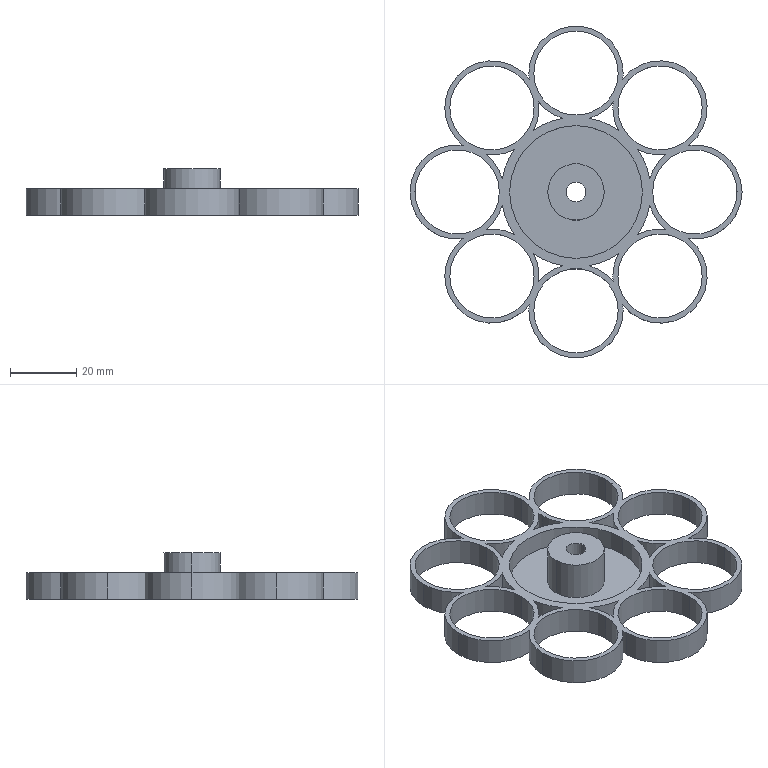Part | SolidWorks | features ICE 2, Extrusion 1 | 1 solid | 67 faces | box 100 x 100 x 14 mm | volume 15045 mm3 | cylinder 63 | plane 4 | commonest cylinder face diameters 28.4 x33 25.4 x16 45.139 x8 6 x2 17 x2 40 x2